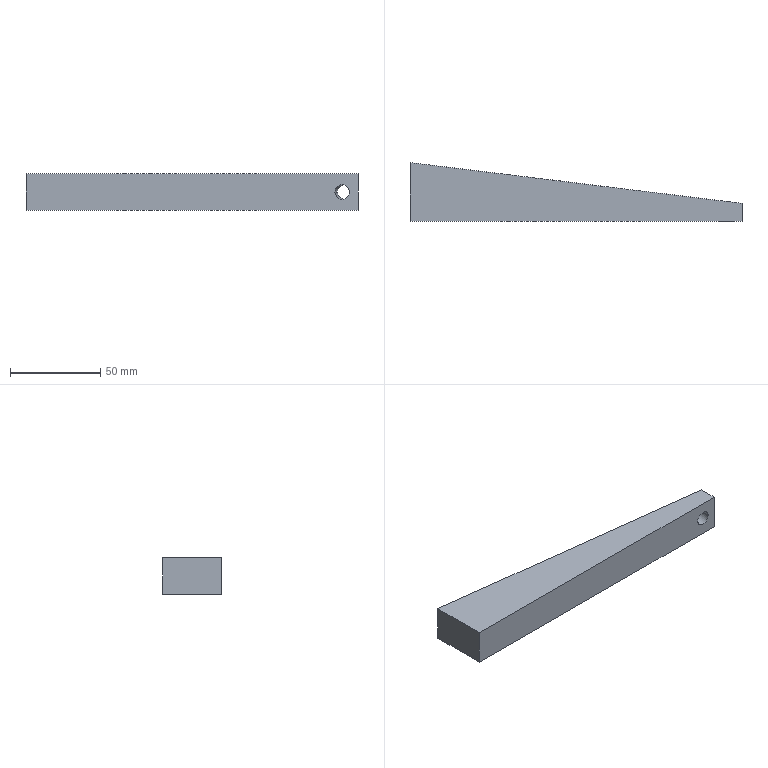Part | SolidWorks | features Extrusion 1, ICE 1, LPattern 1 | 1 solid | 11 faces | box 184 x 32.592 x 20 mm | volume 77063 mm3 | plane 7 | cylinder 4 | commonest cylinder face diameters 8 x4
STEP:
#1=CARTESIAN_POINT('',(9.965,16.256,10.));
#2=VERTEX_POINT('',#1);
#3=CARTESIAN_POINT('',(2.025,17.231,10.));
#4=VERTEX_POINT('',#3);
#5=CARTESIAN_POINT('',(5.995,16.744,10.));
#6=DIRECTION('',(0.1219,0.9925,0.));
#7=DIRECTION('',(-0.9925,0.1219,0.));
#8=AXIS2_PLACEMENT_3D('',#5,#6,#7);
#9=CIRCLE('',#8,4.);
#10=EDGE_CURVE('',#2,#4,#9,.T.);
#11=ORIENTED_EDGE('',*,*,#10,.F.);
#12=CARTESIAN_POINT('',(11.793,31.144,10.));
#13=VERTEX_POINT('',#12);
#14=CARTESIAN_POINT('',(9.965,16.256,10.));
#15=DIRECTION('',(0.1219,0.9925,0.));
#16=VECTOR('',#15,1000.);
#17=LINE('',#14,#16);
#18=EDGE_CURVE('',#2,#13,#17,.T.);
#19=ORIENTED_EDGE('',*,*,#18,.T.);
#20=CARTESIAN_POINT('',(3.853,32.119,10.));
#21=VERTEX_POINT('',#20);
#22=CARTESIAN_POINT('',(7.823,31.632,10.));
#23=DIRECTION('',(0.1219,0.9925,0.));
#24=DIRECTION('',(-0.9925,0.1219,0.));
#25=AXIS2_PLACEMENT_3D('',#22,#23,#24);
#26=CIRCLE('',#25,4.);
#27=EDGE_CURVE('',#13,#21,#26,.T.);
#28=ORIENTED_EDGE('',*,*,#27,.T.);
#29=CARTESIAN_POINT('',(2.025,17.231,10.));
#30=DIRECTION('',(0.1219,0.9925,0.));
#31=VECTOR('',#30,1000.);
#32=LINE('',#29,#31);
#33=EDGE_CURVE('',#4,#21,#32,.T.);
#34=ORIENTED_EDGE('',*,*,#33,.F.);
#35=EDGE_LOOP('',(#11,#19,#28,#34));
#36=FACE_OUTER_BOUND('',#35,.T.);
#37=CARTESIAN_POINT('',(5.995,16.744,10.));
#38=DIRECTION('',(0.1219,0.9925,0.));
#39=DIRECTION('',(-0.9925,0.1219,0.));
#40=AXIS2_PLACEMENT_3D('',#37,#38,#39);
#41=CYLINDRICAL_SURFACE('',#40,4.);
#42=ADVANCED_FACE('',(#36),#41,.F.);
#43=CARTESIAN_POINT('',(179.246,0.,10.));
#44=VERTEX_POINT('',#43);
#45=CARTESIAN_POINT('',(171.186,0.,10.));
#46=VERTEX_POINT('',#45);
#47=CARTESIAN_POINT('',(179.246,0.,10.));
#48=CARTESIAN_POINT('',(179.246,0.,2.));
#49=CARTESIAN_POINT('',(171.186,0.,2.));
#50=CARTESIAN_POINT('',(171.186,0.,10.));
#51=(BOUNDED_CURVE()B_SPLINE_CURVE(3,(#47,#48,#49,#50),.UNSPECIFIED.,.F.,.F.)B_SPLINE_CURVE_WITH_KNOTS((4,4),(0.,3.142),.UNSPECIFIED.)CURVE()GEOMETRIC_REPRESENTATION_ITEM()RATIONAL_B_SPLINE_CURVE((1.,0.3333,0.3333,1.))REPRESENTATION_ITEM(''));
#52=EDGE_CURVE('',#44,#46,#51,.T.);
#53=ORIENTED_EDGE('',*,*,#52,.F.);
#54=CARTESIAN_POINT('',(180.526,10.427,10.));
#55=VERTEX_POINT('',#54);
#56=CARTESIAN_POINT('',(178.698,-4.462,10.));
#57=DIRECTION('',(0.1219,0.9925,0.));
#58=VECTOR('',#57,1000.);
#59=LINE('',#56,#58);
#60=EDGE_CURVE('',#44,#55,#59,.T.);
#61=ORIENTED_EDGE('',*,*,#60,.T.);
#62=CARTESIAN_POINT('',(172.586,11.401,10.));
#63=VERTEX_POINT('',#62);
#64=CARTESIAN_POINT('',(176.556,10.914,10.));
#65=DIRECTION('',(0.1219,0.9925,0.));
#66=DIRECTION('',(-0.9925,0.1219,0.));
#67=AXIS2_PLACEMENT_3D('',#64,#65,#66);
#68=CIRCLE('',#67,4.);
#69=EDGE_CURVE('',#55,#63,#68,.T.);
#70=ORIENTED_EDGE('',*,*,#69,.T.);
#71=CARTESIAN_POINT('',(170.758,-3.487,10.));
#72=DIRECTION('',(0.1219,0.9925,0.));
#73=VECTOR('',#72,1000.);
#74=LINE('',#71,#73);
#75=EDGE_CURVE('',#46,#63,#74,.T.);
#76=ORIENTED_EDGE('',*,*,#75,.F.);
#77=EDGE_LOOP('',(#53,#61,#70,#76));
#78=FACE_OUTER_BOUND('',#77,.T.);
#79=CARTESIAN_POINT('',(174.728,-3.974,10.));
#80=DIRECTION('',(0.1219,0.9925,0.));
#81=DIRECTION('',(-0.9925,0.1219,0.));
#82=AXIS2_PLACEMENT_3D('',#79,#80,#81);
#83=CYLINDRICAL_SURFACE('',#82,4.);
#84=ADVANCED_FACE('',(#78),#83,.F.);
#85=CARTESIAN_POINT('',(0.,32.592,0.));
#86=VERTEX_POINT('',#85);
#87=CARTESIAN_POINT('',(0.,0.,0.));
#88=VERTEX_POINT('',#87);
#89=CARTESIAN_POINT('',(0.,0.,0.));
#90=DIRECTION('',(0.,-1.,0.));
#91=VECTOR('',#90,1000.);
#92=LINE('',#89,#91);
#93=EDGE_CURVE('',#86,#88,#92,.T.);
#94=ORIENTED_EDGE('',*,*,#93,.T.);
#95=CARTESIAN_POINT('',(0.,0.,20.));
#96=VERTEX_POINT('',#95);
#97=CARTESIAN_POINT('',(0.,0.,20.));
#98=DIRECTION('',(0.,0.,-1.));
#99=VECTOR('',#98,1000.);
#100=LINE('',#97,#99);
#101=EDGE_CURVE('',#96,#88,#100,.T.);
#102=ORIENTED_EDGE('',*,*,#101,.F.);
#103=CARTESIAN_POINT('',(0.,32.592,20.));
#104=VERTEX_POINT('',#103);
#105=CARTESIAN_POINT('',(0.,0.,20.));
#106=DIRECTION('',(0.,-1.,0.));
#107=VECTOR('',#106,1000.);
#108=LINE('',#105,#107);
#109=EDGE_CURVE('',#104,#96,#108,.T.);
#110=ORIENTED_EDGE('',*,*,#109,.F.);
#111=CARTESIAN_POINT('',(0.,32.592,20.));
#112=DIRECTION('',(0.,0.,-1.));
#113=VECTOR('',#112,1000.);
#114=LINE('',#111,#113);
#115=EDGE_CURVE('',#104,#86,#114,.T.);
#116=ORIENTED_EDGE('',*,*,#115,.T.);
#117=EDGE_LOOP('',(#94,#102,#110,#116));
#118=FACE_OUTER_BOUND('',#117,.T.);
#119=CARTESIAN_POINT('',(0.,0.,20.));
#120=DIRECTION('',(1.,0.,0.));
#121=DIRECTION('',(0.,0.,-1.));
#122=AXIS2_PLACEMENT_3D('',#119,#120,#121);
#123=PLANE('',#122);
#124=ADVANCED_FACE('',(#118),#123,.F.);
#125=CARTESIAN_POINT('',(171.186,0.,10.));
#126=CARTESIAN_POINT('',(171.186,0.,18.));
#127=CARTESIAN_POINT('',(179.246,0.,18.));
#128=CARTESIAN_POINT('',(179.246,0.,10.));
#129=(BOUNDED_CURVE()B_SPLINE_CURVE(3,(#125,#126,#127,#128),.UNSPECIFIED.,.F.,.F.)B_SPLINE_CURVE_WITH_KNOTS((4,4),(3.142,6.283),.UNSPECIFIED.)CURVE()GEOMETRIC_REPRESENTATION_ITEM()RATIONAL_B_SPLINE_CURVE((1.,0.3333,0.3333,1.))REPRESENTATION_ITEM(''));
#130=EDGE_CURVE('',#46,#44,#129,.T.);
#131=ORIENTED_EDGE('',*,*,#130,.T.);
#132=ORIENTED_EDGE('',*,*,#52,.T.);
#133=EDGE_LOOP('',(#131,#132));
#134=FACE_BOUND('',#133,.T.);
#135=CARTESIAN_POINT('',(184.,0.,0.));
#136=VERTEX_POINT('',#135);
#137=CARTESIAN_POINT('',(0.,0.,0.));
#138=DIRECTION('',(1.,0.,0.));
#139=VECTOR('',#138,1000.);
#140=LINE('',#137,#139);
#141=EDGE_CURVE('',#88,#136,#140,.T.);
#142=ORIENTED_EDGE('',*,*,#141,.T.);
#143=CARTESIAN_POINT('',(184.,0.,20.));
#144=VERTEX_POINT('',#143);
#145=CARTESIAN_POINT('',(184.,0.,20.));
#146=DIRECTION('',(0.,0.,-1.));
#147=VECTOR('',#146,1000.);
#148=LINE('',#145,#147);
#149=EDGE_CURVE('',#144,#136,#148,.T.);
#150=ORIENTED_EDGE('',*,*,#149,.F.);
#151=CARTESIAN_POINT('',(0.,0.,20.));
#152=DIRECTION('',(1.,0.,0.));
#153=VECTOR('',#152,1000.);
#154=LINE('',#151,#153);
#155=EDGE_CURVE('',#96,#144,#154,.T.);
#156=ORIENTED_EDGE('',*,*,#155,.F.);
#157=ORIENTED_EDGE('',*,*,#101,.T.);
#158=EDGE_LOOP('',(#142,#150,#156,#157));
#159=FACE_OUTER_BOUND('',#158,.T.);
#160=CARTESIAN_POINT('',(0.,0.,20.));
#161=DIRECTION('',(0.,1.,0.));
#162=DIRECTION('',(0.,0.,1.));
#163=AXIS2_PLACEMENT_3D('',#160,#161,#162);
#164=PLANE('',#163);
#165=ADVANCED_FACE('',(#134,#159),#164,.F.);
#166=CARTESIAN_POINT('',(184.,10.,0.));
#167=VERTEX_POINT('',#166);
#168=CARTESIAN_POINT('',(184.,0.,0.));
#169=DIRECTION('',(0.,1.,0.));
#170=VECTOR('',#169,1000.);
#171=LINE('',#168,#170);
#172=EDGE_CURVE('',#136,#167,#171,.T.);
#173=ORIENTED_EDGE('',*,*,#172,.T.);
#174=CARTESIAN_POINT('',(184.,10.,20.));
#175=VERTEX_POINT('',#174);
#176=CARTESIAN_POINT('',(184.,10.,20.));
#177=DIRECTION('',(0.,0.,-1.));
#178=VECTOR('',#177,1000.);
#179=LINE('',#176,#178);
#180=EDGE_CURVE('',#175,#167,#179,.T.);
#181=ORIENTED_EDGE('',*,*,#180,.F.);
#182=CARTESIAN_POINT('',(184.,0.,20.));
#183=DIRECTION('',(0.,1.,0.));
#184=VECTOR('',#183,1000.);
#185=LINE('',#182,#184);
#186=EDGE_CURVE('',#144,#175,#185,.T.);
#187=ORIENTED_EDGE('',*,*,#186,.F.);
#188=ORIENTED_EDGE('',*,*,#149,.T.);
#189=EDGE_LOOP('',(#173,#181,#187,#188));
#190=FACE_OUTER_BOUND('',#189,.T.);
#191=CARTESIAN_POINT('',(184.,0.,20.));
#192=DIRECTION('',(-1.,0.,0.));
#193=DIRECTION('',(0.,0.,1.));
#194=AXIS2_PLACEMENT_3D('',#191,#192,#193);
#195=PLANE('',#194);
#196=ADVANCED_FACE('',(#190),#195,.F.);
#197=CARTESIAN_POINT('',(7.823,31.632,10.));
#198=DIRECTION('',(0.1219,0.9925,0.));
#199=DIRECTION('',(-0.9925,0.1219,0.));
#200=AXIS2_PLACEMENT_3D('',#197,#198,#199);
#201=CIRCLE('',#200,4.);
#202=EDGE_CURVE('',#21,#13,#201,.T.);
#203=ORIENTED_EDGE('',*,*,#202,.F.);
#204=ORIENTED_EDGE('',*,*,#27,.F.);
#205=EDGE_LOOP('',(#203,#204));
#206=FACE_BOUND('',#205,.T.);
#207=CARTESIAN_POINT('',(176.556,10.914,10.));
#208=DIRECTION('',(0.1219,0.9925,0.));
#209=DIRECTION('',(-0.9925,0.1219,0.));
#210=AXIS2_PLACEMENT_3D('',#207,#208,#209);
#211=CIRCLE('',#210,4.);
#212=EDGE_CURVE('',#63,#55,#211,.T.);
#213=ORIENTED_EDGE('',*,*,#212,.F.);
#214=ORIENTED_EDGE('',*,*,#69,.F.);
#215=EDGE_LOOP('',(#213,#214));
#216=FACE_BOUND('',#215,.T.);
#217=CARTESIAN_POINT('',(184.,10.,0.));
#218=DIRECTION('',(-0.9925,0.1219,0.));
#219=VECTOR('',#218,1000.);
#220=LINE('',#217,#219);
#221=EDGE_CURVE('',#167,#86,#220,.T.);
#222=ORIENTED_EDGE('',*,*,#221,.T.);
#223=ORIENTED_EDGE('',*,*,#115,.F.);
#224=CARTESIAN_POINT('',(184.,10.,20.));
#225=DIRECTION('',(-0.9925,0.1219,0.));
#226=VECTOR('',#225,1000.);
#227=LINE('',#224,#226);
#228=EDGE_CURVE('',#175,#104,#227,.T.);
#229=ORIENTED_EDGE('',*,*,#228,.F.);
#230=ORIENTED_EDGE('',*,*,#180,.T.);
#231=EDGE_LOOP('',(#222,#223,#229,#230));
#232=FACE_OUTER_BOUND('',#231,.T.);
#233=CARTESIAN_POINT('',(184.,10.,20.));
#234=DIRECTION('',(-0.1219,-0.9925,0.));
#235=DIRECTION('',(0.9925,-0.1219,0.));
#236=AXIS2_PLACEMENT_3D('',#233,#234,#235);
#237=PLANE('',#236);
#238=ADVANCED_FACE('',(#206,#216,#232),#237,.F.);
#239=ORIENTED_EDGE('',*,*,#109,.T.);
#240=ORIENTED_EDGE('',*,*,#155,.T.);
#241=ORIENTED_EDGE('',*,*,#186,.T.);
#242=ORIENTED_EDGE('',*,*,#228,.T.);
#243=EDGE_LOOP('',(#239,#240,#241,#242));
#244=FACE_OUTER_BOUND('',#243,.T.);
#245=CARTESIAN_POINT('',(0.,0.,20.));
#246=DIRECTION('',(0.,0.,-1.));
#247=DIRECTION('',(-1.,0.,0.));
#248=AXIS2_PLACEMENT_3D('',#245,#246,#247);
#249=PLANE('',#248);
#250=ADVANCED_FACE('',(#244),#249,.F.);
#251=ORIENTED_EDGE('',*,*,#93,.F.);
#252=ORIENTED_EDGE('',*,*,#221,.F.);
#253=ORIENTED_EDGE('',*,*,#172,.F.);
#254=ORIENTED_EDGE('',*,*,#141,.F.);
#255=EDGE_LOOP('',(#251,#252,#253,#254));
#256=FACE_OUTER_BOUND('',#255,.T.);
#257=CARTESIAN_POINT('',(0.,0.,0.));
#258=DIRECTION('',(0.,0.,-1.));
#259=DIRECTION('',(-1.,0.,0.));
#260=AXIS2_PLACEMENT_3D('',#257,#258,#259);
#261=PLANE('',#260);
#262=ADVANCED_FACE('',(#256),#261,.T.);
#263=ORIENTED_EDGE('',*,*,#60,.F.);
#264=ORIENTED_EDGE('',*,*,#130,.F.);
#265=ORIENTED_EDGE('',*,*,#75,.T.);
#266=ORIENTED_EDGE('',*,*,#212,.T.);
#267=EDGE_LOOP('',(#263,#264,#265,#266));
#268=FACE_OUTER_BOUND('',#267,.T.);
#269=CARTESIAN_POINT('',(174.728,-3.974,10.));
#270=DIRECTION('',(0.1219,0.9925,0.));
#271=DIRECTION('',(-0.9925,0.1219,0.));
#272=AXIS2_PLACEMENT_3D('',#269,#270,#271);
#273=CYLINDRICAL_SURFACE('',#272,4.);
#274=ADVANCED_FACE('',(#268),#273,.F.);
#275=ORIENTED_EDGE('',*,*,#18,.F.);
#276=CARTESIAN_POINT('',(5.995,16.744,10.));
#277=DIRECTION('',(0.1219,0.9925,0.));
#278=DIRECTION('',(-0.9925,0.1219,0.));
#279=AXIS2_PLACEMENT_3D('',#276,#277,#278);
#280=CIRCLE('',#279,4.);
#281=EDGE_CURVE('',#4,#2,#280,.T.);
#282=ORIENTED_EDGE('',*,*,#281,.F.);
#283=ORIENTED_EDGE('',*,*,#33,.T.);
#284=ORIENTED_EDGE('',*,*,#202,.T.);
#285=EDGE_LOOP('',(#275,#282,#283,#284));
#286=FACE_OUTER_BOUND('',#285,.T.);
#287=CARTESIAN_POINT('',(5.995,16.744,10.));
#288=DIRECTION('',(0.1219,0.9925,0.));
#289=DIRECTION('',(-0.9925,0.1219,0.));
#290=AXIS2_PLACEMENT_3D('',#287,#288,#289);
#291=CYLINDRICAL_SURFACE('',#290,4.);
#292=ADVANCED_FACE('',(#286),#291,.F.);
#293=ORIENTED_EDGE('',*,*,#281,.T.);
#294=ORIENTED_EDGE('',*,*,#10,.T.);
#295=EDGE_LOOP('',(#293,#294));
#296=FACE_OUTER_BOUND('',#295,.T.);
#297=CARTESIAN_POINT('',(5.995,16.744,10.));
#298=DIRECTION('',(0.1219,0.9925,0.));
#299=DIRECTION('',(-0.9925,0.1219,0.));
#300=AXIS2_PLACEMENT_3D('',#297,#298,#299);
#301=PLANE('',#300);
#302=ADVANCED_FACE('',(#296),#301,.T.);
#303=CLOSED_SHELL('',(#42,#84,#124,#165,#196,#238,#250,#262,#274,#292,#302));
#304=MANIFOLD_SOLID_BREP('',#303);
#305=CARTESIAN_POINT('',(0.,0.,0.));
#306=DIRECTION('',(0.,0.,1.));
#307=DIRECTION('',(1.,0.,0.));
#308=AXIS2_PLACEMENT_3D('',#305,#306,#307);
#309=(LENGTH_UNIT()NAMED_UNIT(*)SI_UNIT(.MILLI.,.METRE.));
#310=UNCERTAINTY_MEASURE_WITH_UNIT(LENGTH_MEASURE(0.00001),#309,'','');
#311=(NAMED_UNIT(*)PLANE_ANGLE_UNIT()SI_UNIT($,.RADIAN.));
#312=(NAMED_UNIT(*)SI_UNIT($,.STERADIAN.)SOLID_ANGLE_UNIT());
#313=(GEOMETRIC_REPRESENTATION_CONTEXT(3)GLOBAL_UNCERTAINTY_ASSIGNED_CONTEXT((#310))GLOBAL_UNIT_ASSIGNED_CONTEXT((#309,#311,#312))REPRESENTATION_CONTEXT('',''));
#314=ADVANCED_BREP_SHAPE_REPRESENTATION('',(#304,#308),#313);